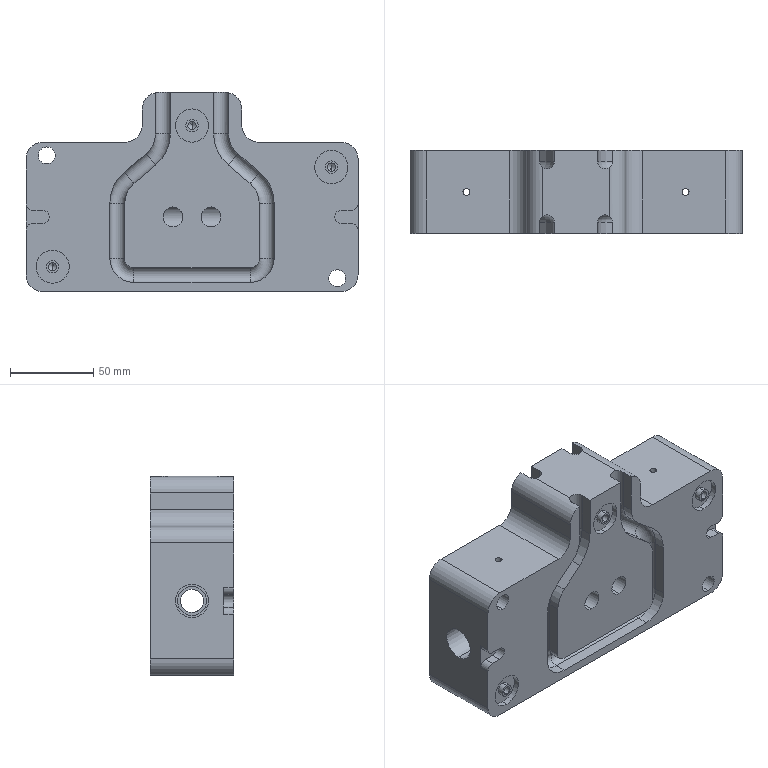Part | STEP file | Manifold-cc | 1 solid | 201 faces | box 200 x 50 x 120 mm | volume 855215 mm3 | cylinder 112 | plane 59 | cone 18 | torus 12 | commonest cylinder face diameters 20 x18 9 x14 5 x10 4.2 x8 6.8 x8 31 x8